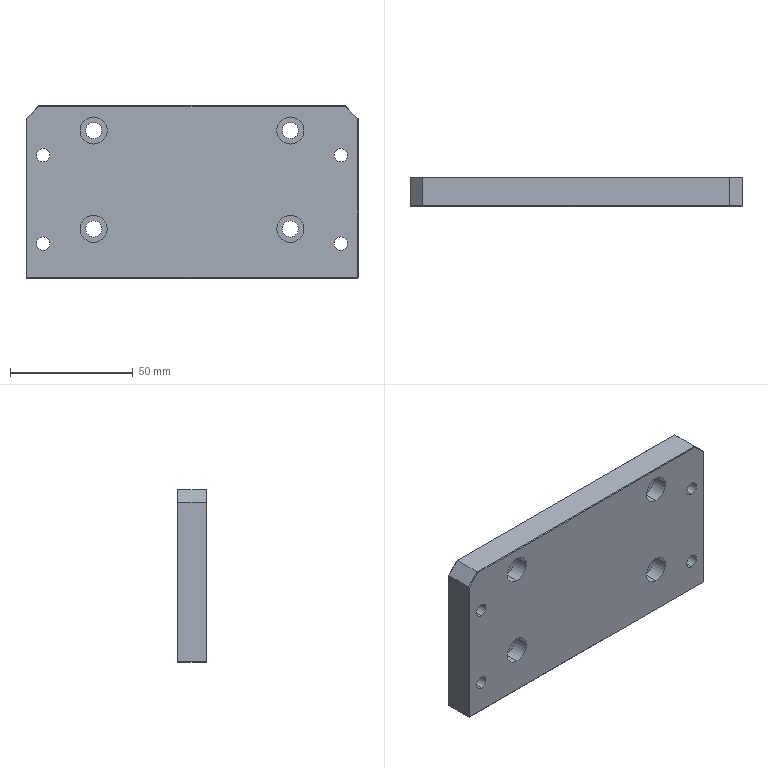Part | STEP file | ND25021-01-JDKM-43-TL | 1 solid | 78 faces | box 135 x 12 x 70 mm | volume 107007 mm3 | cylinder 38 | plane 34 | cone 6 | commonest cylinder face diameters 5.5 x8 6.6 x8 10 x8 11 x8 4.2 x6